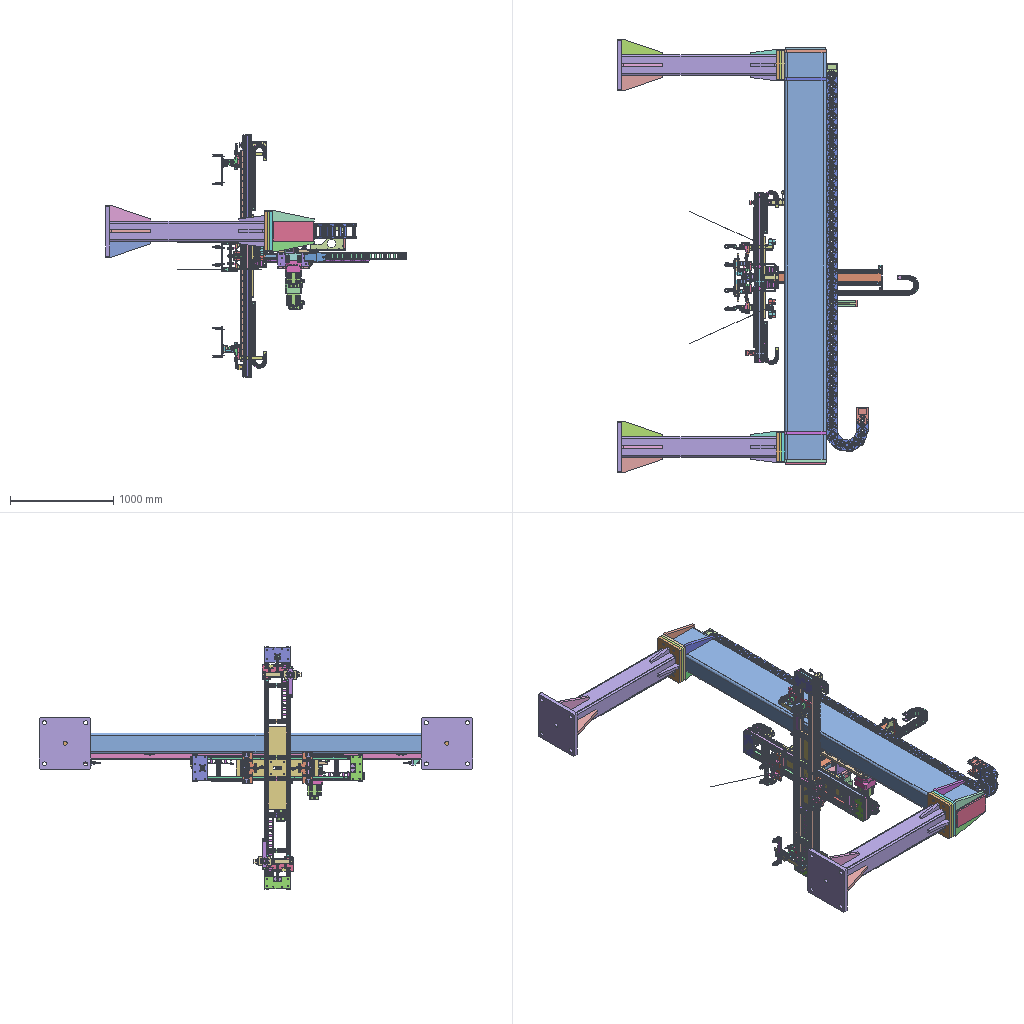Assembly | SolidWorks | 170 different items | 561 placed | box 2915 x 4200 x 2346 mm
Parts list (item | name | quantity | parent item | size | volume | features):
1 | (subassembly) | x2 | - | - | 1868083 mm3 | features InContextFeatHolder 12, ReferencePattern 4, CompositeCurve 2, MirrorCompFeat 1
2 | (subassembly) | x2 | - | - | 1438864 mm3 | features InContextFeatHolder 22, ReferencePattern 3, CompositeCurve 1, MirrorCompFeat 1
3 | (subassembly) | x1 | in 22 | 29 x 32 x 32 mm | 15807 mm3 | -
4 | (subassembly) | x1 | in 22 | 45 x 45 x 34 mm | 25485 mm3 | -
5 | (subassembly) | x1 | in 22 | 45 x 45 x 22 mm | 19865 mm3 | -
6 | (subassembly) | x4 | in 1 | 100.5 x 39 x 24.85 mm | 31183 mm3 | -
7 | (subassembly) | x2 | in 1 | 191 x 54 x 69 mm | 317476 mm3 | -
8 | (subassembly) | x2 | in 21 | 38.735 x 58.5 x 31.374 mm | 22045 mm3 | -
9 | (subassembly) | x2 | in 1 | 179.68 x 29.769 x 35.214 mm | 28072 mm3 | -
10 | (subassembly) | x1 | in 16 | 220 x 170 x 130 mm | 1941272 mm3 | -
11 | (subassembly) | x4 | in 2 | 17 x 70.5 x 19.048 mm | 7303 mm3 | -
12 | (subassembly) | x2 | in 22 | - | 654604 mm3 | -
13 | (subassembly) | x2 | in 22 | 72.4 x 145.352 x 414.628 mm | 469160 mm3 | -
14 | (subassembly) | x1 | in 21 | - | 1169113 mm3 | features ReferencePattern 9, LocalLPattern 1
15 | (subassembly) | x1 | in 20 | - | 15476828 mm3 | -
16 | (subassembly) | x1 | in 21 | 220 x 170 x 130 mm | 1941272 mm3 | -
17 | (subassembly) | x4 | in 2 | 100.5 x 39 x 24.85 mm | 31183 mm3 | -
18 | (subassembly) | x2 | in 2 | 179.229 x 29.769 x 35.214 mm | 28072 mm3 | -
19 | (subassembly) | x2 | in 20 | 26 x 157 x 29.132 mm | 41866 mm3 | -
20 | (subassembly) | x1 | - | - | 164128062 mm3 | features ReferencePattern 3, LocalLPattern 2
21 | (subassembly) | x1 | - | - | 39375353 mm3 | features InContextFeatHolder 40, ReferencePattern 26, LocalLPattern 4, LocalCirPattern 1, MirrorCompFeat 1
22 | (subassembly) | x1 | - | - | 17712446 mm3 | features ReferencePattern 14, InContextFeatHolder 8, Belt 2, LocalCirPattern 2, MirrorCompFeat 1, RefAxis 1
23 | (subassembly) | x4 | in 1 | 17 x 70.5 x 19.048 mm | 7303 mm3 | -
24 | - | x2 | in 18 | 116 x 21 x 21 mm | 16272 mm3 | features BaseBody 1, ICE 1, MoveCopyBody 1, Split 1
25 | - | x2 | in 21 | 23 x 18 x 900 mm | 312541 mm3 | features BaseBody 1, HoleWzd 1, ICE 1, MoveFace 1
26 | - | x4 | in 22 | 15 x 12.5 x 540 mm | 86755 mm3 | features BaseBody 1, HoleWzd 1, ICE 1, MoveFace 1
27 | - | x4 | in 20 | 23 x 18 x 1620 mm | 561456 mm3 | features MoveFace 3, BaseBody 1, HoleWzd 1
28 | - | x4 | in 22 | 15 x 12.5 x 1020 mm | 163723 mm3 | features BaseBody 1, HoleWzd 1, ICE 1, MoveFace 1
29 | - | x2 | in 1 | 34 x 19.5 x 56.8 mm | 30383 mm3 | features BaseBody 1
30 | - | x10 | in 21 | 48 x 26 x 82.6 mm | 80910 mm3 | features BaseBody 1
31 | - | x4 | in 1 | 12 x 42 x 42 mm | 9526 mm3 | features Revolution 5, CirPattern 2, RefAxis 1, RevCut 1
32 | - | x1 | in 21 | 160 x 160 x 283 mm | 4310215 mm3 | features ICE 18, CirPattern 4, Fillet 2, Revolution 2, Chamfer 1, RevCut 1
33 | - | x1 | in 21 | 160 x 160 x 330 mm | 5402193 mm3 | features ICE 18, CirPattern 4, Fillet 2, Revolution 2, Chamfer 1, RevCut 1
34 | - | x1 | in 22 | 54 x 54 x 34.8 mm | 31489 mm3 | features BaseBody 1
35 | - | x4 | in 11 | 12 x 70.5 x 12 mm | 6151 mm3 | features BaseBody 1
36 | - | x2 | in 22 | 60 x 60 x 115 mm | 222679 mm3 | features BaseBody 7
37 | - | x2 | in 8 | 31.47 x 20 x 31.374 mm | 10219 mm3 | features BaseBody 1
38 | - | x2 | in 8 | 33 x 58.5 x 20 mm | 11826 mm3 | features BaseBody 1
39 | - | x12 | in 6, 7 | 4 x 5.4 x 50 mm | 499.042 mm3 | features BaseBody 1
40 | - | x2 | in 9 | 6 x 25 x 22 mm | 1467 mm3 | features BaseBody 1
41 | - | x2 | in 9 | 5 x 11.547 x 10 mm | 331.011 mm3 | features BaseBody 1
42 | - | x2 | in 9 | 108 x 15.5 x 15.5 mm | 6247 mm3 | features BaseBody 1
43 | - | x2 | in 9 | 116 x 21 x 21 mm | 16272 mm3 | features BaseBody 1, ICE 1, MoveCopyBody 1, Split 1
44 | - | x2 | in 21 | 60 x 24 x 205 mm | 179716 mm3 | features BaseBody 1
45 | - | x4 | in 23 | 12 x 70.5 x 12 mm | 6151 mm3 | features BaseBody 1
46 | - | x8 | in 11 | 17 x 4 x 19.048 mm | 576.259 mm3 | features BaseBody 1
47 | - | x8 | in 23 | 17 x 4 x 19.048 mm | 576.259 mm3 | features BaseBody 1
48 | - | x2 | in 19 | 20 x 157 x 20 mm | 38514 mm3 | features BaseBody 1
49 | - | x4 | in 19 | 26 x 6 x 29.132 mm | 1676 mm3 | features BaseBody 1
50 | - | x4 | in 9 | 37.5 x 29.1 x 18.4 mm | 1877 mm3 | features BaseBody 1
51 | - | x1 | in 3 | 13.7 x 32 x 32 mm | 7455 mm3 | features BaseBody 1, ICE 1
52 | - | x1 | in 3 | 13.7 x 32 x 32 mm | 6989 mm3 | features BaseBody 1
53 | - | x1 | in 3 | 5.6 x 31 x 31 mm | 974.208 mm3 | features BaseBody 1
54 | - | x4 | in 3 | 9 x 5 x 5 mm | 97.086 mm3 | features BaseBody 1
55 | - | x1 | in 22 | 45 x 45 x 22 mm | 22602 mm3 | features ICE 4, BaseBody 1
56 | - | x1 | in 4 | 45 x 45 x 34 mm | 25485 mm3 | features BaseBody 1
57 | - | x4 | in 18 | 37.5 x 29.1 x 18.4 mm | 1877 mm3 | features BaseBody 1
58 | - | x4 | in 1, 2 | 33 x 6 x 36 mm | 5895 mm3 | features ICE 2, MoveFace 2, BaseBody 1, HoleWzd 1
59 | - | x2 | in 5, 22 | 45 x 45 x 22 mm | 19865 mm3 | features BaseBody 1, RefAxis 1
60 | - | x4 | in 6 | 50 x 39 x 23.5 mm | 27612 mm3 | features BaseBody 1
61 | - | x4 | in 6 | 21 x 15.4 x 10.1 mm | 1286 mm3 | features BaseBody 1
62 | - | x4 | in 6 | 21 x 15.4 x 10.1 mm | 1286 mm3 | features BaseBody 1
63 | - | x2 | in 7 | 169 x 54 x 69 mm | 316478 mm3 | features BaseBody 1
64 | - | x2 | in 10, 21 | 220 x 170 x 130 mm | 1941272 mm3 | features BaseBody 1
65 | - | x54 | in 12, 13 | 68 x 35.356 x 81.35 mm | 37089 mm3 | features BaseBody 1
66 | - | x23 | in 14 | 72.6 x 45.28 x 91.28 mm | 47406 mm3 | features BaseBody 1
67 | - | x40 | in 15 | 145 x 107 x 206.999 mm | 368273 mm3 | features BaseBody 1
68 | - | x4 | in 17 | 50 x 39 x 23.5 mm | 27612 mm3 | features BaseBody 1
69 | - | x4 | in 12, 13 | 72.4 x 35.35 x 67.662 mm | 29898 mm3 | features BaseBody 1
70 | - | x4 | in 12, 13 | 72.4 x 35.35 x 67.664 mm | 31284 mm3 | features BaseBody 1
71 | - | x1 | in 14 | 73.47 x 44.999 x 83.497 mm | 38091 mm3 | features BaseBody 1
72 | - | x1 | in 14 | 73.47 x 44.999 x 83.497 mm | 40679 mm3 | features BaseBody 1
73 | - | x1 | in 15 | 144 x 107 x 180 mm | 372084 mm3 | features BaseBody 1
74 | - | x1 | in 15 | 144 x 107 x 180 mm | 373805 mm3 | features BaseBody 1
75 | - | x2 | in 1 | 50 x 50 x 10 mm | 14543 mm3 | features BaseBody 1, RefAxis 1
76 | - | x2 | in 1 | 50 x 12 x 10 mm | 5397 mm3 | features BaseBody 1, HoleWzd 1, ICE 1
77 | - | x4 | in 17 | 21 x 15.4 x 10.1 mm | 1286 mm3 | features BaseBody 1
78 | - | x4 | in 17 | 21 x 15.4 x 10.1 mm | 1286 mm3 | features BaseBody 1
79 | - | x2 | in 2 | 50 x 50 x 10 mm | 14543 mm3 | features BaseBody 1, RefAxis 1
80 | - | x2 | in 2 | 50 x 12 x 10 mm | 5397 mm3 | features BaseBody 1, HoleWzd 1, ICE 1
81 | - | x1 | in 21 | 142 x 202 x 99 mm | 619754 mm3 | features BaseBody 1
82 | - | x1 | in 20 | 2009 x 24 x 24 mm | 1024177 mm3 | features ICE 10, BaseBody 1, LPattern 1, MoveFace 1
83 | - | x8 | in 21 | - | - | features RefSurface 9
84 | - | x4 | in 21 | - | - | features RefSurface 9
85 | - | x2 | in 21 | 13.344 x 9 x 13.344 mm | 1017 mm3 | features BaseBody 1
86 | - | x2 | in 21 | - | - | features RefSurface 1
87 | - | x2 | in 20 | 1570 x 500 x 500 mm | 29641235 mm3 | features ICE 3, Chamfer 2, CirPattern 2, HoleWzd 2, Split 2, CombineBodies 1, Rib 1, WeldMemberFeat 1, WeldmentFeature 1
88 | - | x1 | in 20 | 4040 x 400 x 430 mm | 79794691 mm3 | features HoleWzd 6, ICE 4, MirrorSolid 3, Chamfer 2, EndCap 2, Cut 1, MirrorPattern 1, WeldMemberFeat 1, WeldmentFeature 1
89 | - | x2 | in 20 | 300 x 20 x 400 mm | 2385381 mm3 | features Chamfer 1, Extrusion 1, HoleWzd 1
90 | - | x2 | in 20 | 90 x 100 x 110 mm | 460863 mm3 | features HoleWzd 3, ICE 2, Extrusion 1, MirrorSolid 1
91 | - | x2 | in 20 | 28 x 5 x 100 mm | 4922 mm3 | features BossThin 1, ExtruThin 1, HoleWzd 1, MirrorSolid 1
92 | - | x1 | in 21 | 600 x 25 x 300 mm | 3745145 mm3 | features HoleWzd 11, Cut 2, Chamfer 1, Extrusion 1
93 | - | x2 | in 20, 21 | 1008 x 24 x 24 mm | 511477 mm3 | features BaseBody 1
94 | - | x1 | in 21 | 248 x 60 x 12 mm | 176365 mm3 | features HoleWzd 2, Chamfer 1, Extrusion 1
95 | - | x1 | in 21 | 25 x 60 x 12 mm | 15515 mm3 | features HoleWzd 2, Chamfer 1, Extrusion 1
96 | - | x1 | in 21 | 25 x 98 x 142 mm | 49886 mm3 | features HoleWzd 2, BreakCorner 1, FlatPattern 1, SMBaseFlange 1, SheetMetal 1
97 | - | x1 | in 21 | 300 x 25 x 300 mm | 1546097 mm3 | features HoleWzd 9, Cut 2, Chamfer 1, Extrusion 1
98 | - | x2 | in 21 | 200 x 180 x 12 mm | 261071 mm3 | features HoleWzd 4, MirrorPattern 2, Chamfer 1, Cut 1, Extrusion 1
99 | - | x2 | in 21 | 50 x 25 x 15 mm | 15237 mm3 | features HoleWzd 2, Chamfer 1, Extrusion 1
100 | - | x1 | in 21 | 1125 x 200 x 236 mm | 3630332 mm3 | features ICE 7, HoleWzd 5, Chamfer 2, Fillet 2, Cut 1, EndCap 1, MirrorPattern 1, MoveFace 1, WeldMemberFeat 1, WeldmentFeature 1
101 | - | x2 | in 21 | 50 x 25 x 15 mm | 15782 mm3 | features Chamfer 1, Extrusion 1, HoleWzd 1
102 | - | x1 | in 21 | 800 x 20 x 800 mm | 6619888 mm3 | features HoleWzd 3, Chamfer 1, Cut 1, Extrusion 1, Fillet 1
103 | - | x1 | in 21 | 135 x 25 x 300 mm | 964423 mm3 | features HoleWzd 3, Cut 1, Extrusion 1, MirrorPattern 1
104 | - | x4 | in 2 | 34 x 19.5 x 56.8 mm | 30383 mm3 | features BaseBody 1
105 | - | x1 | in 21 | 135 x 25 x 300 mm | 964423 mm3 | features MirrorStock 1
106 | - | x1 | in 21 | 340 x 60 x 12 mm | 241410 mm3 | features HoleWzd 3, Chamfer 1, Extrusion 1
107 | - | x1 | in 21 | 80 x 75 x 10 mm | 45981 mm3 | features HoleWzd 2, Chamfer 1, Cut 1, Extrusion 1
108 | - | x1 | in 21 | 248 x 323 x 12 mm | 393029 mm3 | features HoleWzd 2, ICE 2, Extrusion 1, Fillet 1
109 | - | x2 | in 21 | 25 x 34.5 x 20 mm | 1892 mm3 | features BreakCorner 1, FlatPattern 1, HoleWzd 1, ICE 1, SMBaseFlange 1, SheetMetal 1
110 | - | x1 | in 21 | 15 x 62.5 x 20 mm | 2923 mm3 | features BreakCorner 1, FlatPattern 1, HoleWzd 1, SMBaseFlange 1, SheetMetal 1
111 | - | x1 | in 21 | 28 x 5 x 800 mm | 39502 mm3 | features BossThin 1, ExtruThin 1, HoleWzd 1, MirrorSolid 1
112 | - | x1 | in 21 | 12 x 37 x 20 mm | 1356 mm3 | features BreakCorner 1, FlatPattern 1, HoleWzd 1, SMBaseFlange 1, SheetMetal 1
113 | - | x1 | in 21 | 25 x 25 x 13 mm | 5523 mm3 | features Extrusion 1, HoleWzd 1
114 | - | x4 | in 22 | 540 x 12 x 40 mm | 251867 mm3 | features HoleWzd 3, LPattern 2, Chamfer 1, Extrusion 1
115 | - | x4 | in 2 | 12 x 42 x 42 mm | 9526 mm3 | features Revolution 5, CirPattern 2, RefAxis 1, RevCut 1
116 | - | x4 | in 22 | 1020 x 20 x 40 mm | 797316 mm3 | features HoleWzd 3, LPattern 2, Chamfer 1, Extrusion 1
117 | - | x1 | in 22 | - | 6888889 mm3 | features WeldMemberFeat 1, WeldmentFeature 1
118 | - | x2 | in 22 | 250 x 12 x 117.5 mm | 341494 mm3 | features HoleWzd 4, Chamfer 1, Extrusion 1
119 | - | x1 | in 22 | 50 x 34 x 12 mm | 19690 mm3 | features Extrusion 1, HoleWzd 1, MirrorPattern 1
120 | - | x2 | in 22 | 50 x 79 x 12 mm | 40495 mm3 | features HoleWzd 3, Chamfer 1, Extrusion 1
121 | - | x4 | in 22 | 10 x 10 x 70 mm | 5498 mm3 | features Extrusion 1
122 | - | x2 | in 22 | 50 x 74 x 12 mm | 31467 mm3 | features Extrusion 1, HoleWzd 1, ICE 1, MirrorPattern 1
123 | - | x2 | in 22 | 250 x 12 x 145 mm | 416706 mm3 | features Cut 2, HoleWzd 2, Chamfer 1, Extrusion 1
124 | - | x1 | in 22 | 10 x 10 x 58 mm | 4483 mm3 | features ICE 2, MirrorPattern 2, Extrusion 1, RefAxis 1
125 | - | x1 | in 22 | 50 x 34 x 12 mm | 19690 mm3 | features Extrusion 1, HoleWzd 1, MirrorPattern 1
126 | - | x8 | in 17 | 4 x 5.4 x 50 mm | 499.042 mm3 | features BaseBody 1
127 | - | x1 | in 22 | 10 x 10 x 98 mm | 7613 mm3 | features ICE 2, MirrorPattern 2, Extrusion 1, RefAxis 1
128 | - | x8 | in 22 | 40 x 3 x 80 mm | 9527 mm3 | features Fillet 2, Extrusion 1
129 | - | x1 | in 22 | 16 x 16 x 87 mm | 9059 mm3 | features ICE 2, Extrusion 1, HoleWzd 1, Revolution 1
130 | - | x4 | in 1 | 25 x 10 x 25 mm | 3874 mm3 | features HoleWzd 2, Chamfer 1, Extrusion 1
131 | - | x2 | in 1 | 26 x 80 x 22 mm | 22644 mm3 | features Chamfer 2, Cut 2, Extrusion 1, HoleWzd 1, ICE 1, MirrorPattern 1
132 | - | x4 | in 1 | 35 x 60 x 40 mm | 35844 mm3 | features Chamfer 2, HoleWzd 2, Extrusion 1, ICE 1
133 | - | x2 | in 1 | 80 x 300 x 12 mm | 155894 mm3 | features Cut 3, HoleWzd 3, Chamfer 2, CirPattern 1, Extrusion 1, Fillet 1
134 | - | x2 | in 1 | 80 x 333.5 x 12 mm | 174640 mm3 | features Chamfer 2, Cut 2, HoleWzd 2, Extrusion 1, Fillet 1
135 | - | x2 | in 1 | 46 x 15 x 50 mm | 17863 mm3 | features Chamfer 4, Extrusion 1, HoleWzd 1, ICE 1
136 | - | x2 | in 1 | 20 x 50 x 10 mm | 7631 mm3 | features Chamfer 1, Extrusion 1, HoleWzd 1
137 | - | x2 | in 18 | 6 x 25 x 22 mm | 1467 mm3 | features BaseBody 1
138 | - | x2 | in 1 | 20 x 235 x 20 mm | 73572 mm3 | features ICE 3, Chamfer 1, Extrusion 1
139 | - | x4 | in 1 | 95 x 20 x 80 mm | 71658 mm3 | features ICE 2, Chamfer 1, Extrusion 1, Fillet 1, HoleWzd 1
140 | - | x4 | in 1 | 15 x 35 x 40 mm | 15250 mm3 | features Chamfer 1, Extrusion 1, HoleWzd 1
141 | - | x4 | in 1 | 27 x 35 x 80 mm | 44069 mm3 | features Chamfer 2, HoleWzd 2, Extrusion 1, ICE 1
142 | - | x4 | in 1 | 35 x 12 x 34.943 mm | 6766 mm3 | features HoleWzd 2, Chamfer 1, Extrusion 1, ICE 1, MirrorPattern 1
143 | - | x2 | in 1 | 30 x 37.5 x 36 mm | 19999 mm3 | features HoleWzd 2, Chamfer 1, ExtruThin 1
144 | - | x8 | in 1 | 17.5 x 30 x 12 mm | 2171 mm3 | features Extrusion 1, Fillet 1, HoleWzd 1, ICE 1
145 | - | x4 | in 1, 2 | 113 x 30 x 232 mm | 30522 mm3 | features BreakCorner 1, FlatPattern 1, SMBaseFlange 1, SheetMetal 1
146 | - | x4 | in 1 | 35 x 35 x 20 mm | 13186 mm3 | features HoleWzd 3, Chamfer 1, Extrusion 1, ICE 1
147 | - | x2 | in 1 | 300 x 140 x 20 mm | 458590 mm3 | features HoleWzd 8, Chamfer 5, Cut 4, Fillet 4, ICE 3, Extrusion 1
148 | - | x2 | in 18 | 5 x 11.547 x 10 mm | 331.011 mm3 | features BaseBody 1
149 | - | x5 | in 1, 21 | 25 x 25 x 23 mm | 9481 mm3 | features Extrusion 1, HoleWzd 1
150 | - | x4 | in 2 | 35 x 35 x 20 mm | 13186 mm3 | features HoleWzd 3, Chamfer 1, Extrusion 1, ICE 1
151 | - | x2 | in 2 | 20 x 50 x 10 mm | 7631 mm3 | features Chamfer 1, Extrusion 1, HoleWzd 1
152 | - | x2 | in 2 | 46 x 15 x 50 mm | 17863 mm3 | features Chamfer 4, Extrusion 1, HoleWzd 1, ICE 1
153 | - | x2 | in 2 | 26 x 80 x 22 mm | 22644 mm3 | features Chamfer 2, Cut 2, Extrusion 1, HoleWzd 1, ICE 1, MirrorPattern 1
154 | - | x2 | in 2 | 20 x 300 x 20 mm | 93992 mm3 | features ICE 3, Chamfer 1, Extrusion 1
155 | - | x2 | in 2 | 300 x 140 x 20 mm | 435356 mm3 | features HoleWzd 7, Chamfer 4, Cut 4, Fillet 3, ICE 2, Extrusion 1
156 | - | x2 | in 2 | 40 x 300 x 12 mm | 108008 mm3 | features Cut 3, Chamfer 2, HoleWzd 2, ICE 2, Extrusion 1, Fillet 1
157 | - | x4 | in 2 | 35 x 56.7 x 40 mm | 34458 mm3 | features Chamfer 2, HoleWzd 2, Extrusion 1, ICE 1
158 | - | x2 | in 2 | 30 x 37.5 x 36 mm | 19999 mm3 | features HoleWzd 2, Chamfer 1, ExtruThin 1
159 | - | x2 | in 18 | 108 x 15.5 x 15.5 mm | 6247 mm3 | features BaseBody 1
160 | - | x4 | in 2 | 35 x 12 x 34.943 mm | 6766 mm3 | features HoleWzd 2, Chamfer 1, Extrusion 1, ICE 1, MirrorPattern 1
161 | - | x4 | in 2 | 15 x 35 x 40 mm | 15250 mm3 | features Chamfer 1, Extrusion 1, HoleWzd 1
162 | - | x4 | in 2 | 95 x 20 x 80 mm | 71658 mm3 | features ICE 2, Chamfer 1, Extrusion 1, Fillet 1, HoleWzd 1
163 | - | x4 | in 2 | 56.8 x 38 x 28 mm | 56349 mm3 | features Chamfer 1, Cut 1, Extrusion 1
164 | - | x4 | in 2 | 27 x 35 x 80 mm | 44069 mm3 | features Chamfer 2, HoleWzd 2, Extrusion 1, ICE 1
165 | - | x8 | in 2 | 17.5 x 30 x 12 mm | 2171 mm3 | features Extrusion 1, Fillet 1, HoleWzd 1, ICE 1
166 | - | x8 | in 21 | - | - | features RefSurface 2
167 | - | x2 | in 22 | 63.089 x 175.904 x 146.235 mm | 489456 mm3 | features BaseBody 2
168 | - | x3 | in 20 | 26.2 x 15.5 x 20.7 mm | 2180 mm3 | features BaseBody 1
169 | - | x1 | in 21 | 26.2 x 15.5 x 20.7 mm | 2180 mm3 | features BaseBody 1
170 | - | x2 | in 21 | 100 x 100 x 76 mm | 350240 mm3 | features ICE 3, Chamfer 2, CirPattern 2, HoleWzd 1, RefAxis 1, Revolution 1
Mates (type | each side: item.copy, entity, surface, feature), first 385 of 538 lines:
In the top assembly
Width | 155.1 face plane Boss-Extrude 1 | 155.1 face plane Boss-Extrude 1 | 117.1 face plane Aluminium Profile 40 X 80L X R0.3(1) | 117.1 face plane Aluminium Profile 40 X 80L X R0.3(1)
Coincident | 26.1 face plane 输入1 | 104.1 face plane 输入1
DistanceDim | assembly plane | 87.1 face plane Boss-Extrude 1
DistanceDim | assembly plane | 87.1 face plane Gb/6728-1986方形空心型钢 200 X 200 X 10(1)
Parallel | 88.1 face plane Gb/6728-1986矩形空心型钢 400 X 200 X 12(1) | assembly plane
Width | 30.1 face plane 输入1 | 30.1 face plane 输入1 | 27.1 face plane 输入1 | 27.1 face plane 输入1
Width | 30.2 face plane 输入1 | 30.2 face plane 输入1 | 27.2 face plane 输入1 | 27.2 face plane 输入1
Coincident | 102.1 face plane Boss-Extrude 1 | 117.1 face plane Aluminium Profile 40 X 80L X R0.3(1)
Width | 117.1 face plane Aluminium Profile 40 X 80L X R0.3(1) | 117.1 face plane Aluminium Profile 40 X 80L X R0.3(1) | 102.1 face plane Boss-Extrude 1 | 102.1 face plane Boss-Extrude 1 | 2 times
Parallel | 82.1 face plane 输入1 | 8.1 plane
LimitDistanceDim | 92.1 face plane Boss-Extrude 1 | 88.1 face plane Boss-Extrude 3
LimitDistanceDim | 155.2 face plane Boss-Extrude 1 | 123.1 face plane Boss-Extrude 1
Parallel | assembly face | 87.1 face plane Boss-Extrude 1
Width | assembly face | assembly face | 117.1 face plane Aluminium Profile 40 X 80L X R0.3(1) | 117.1 face plane Aluminium Profile 40 X 80L X R0.3(1) | 2 times
Coincident | 28.1 face plane 输入1 | 29.1 face plane 输入1
Width | 147.1 face plane Boss-Extrude 1 | 147.1 face plane Boss-Extrude 1 | 116.1 face plane Boss-Extrude 1 | 116.2 face plane Boss-Extrude 1
LimitDistanceDim | 147.1 face plane Boss-Extrude 1 | 116.1 face plane Boss-Extrude 1
Coincident | 87.1 face plane Gb/6728-1986方形空心型钢 200 X 200 X 10(1) | assembly plane
Coincident | 27.1 face plane 输入1 | 30.1 face plane 输入1
In subassembly 1
Coincident | 147.2 face plane Cut-Extrude 2 | 143.1 face plane Extrude-薄壁1
Width | 147.2 face plane Boss-Extrude 1 | 147.2 face plane Boss-Extrude 1 | 143.1 face plane Extrude-薄壁1 | 143.1 face plane Extrude-薄壁1
DistanceDim | 143.1 face plane Extrude-薄壁1 | 147.2 face plane Boss-Extrude 1
Coincident | 29.2 face plane 输入1 | 147.2 face plane Cut-Extrude 1
Width | 143.1 face plane Extrude-薄壁1 | 143.1 face plane Extrude-薄壁1 | 58.1 face plane 输入1 | 58.1 face plane 输入1
Width | 29.2 face plane 输入1 | 29.2 face plane 输入1 | 147.2 face plane Cut-Extrude 1 | 147.2 face plane Cut-Extrude 1
Width | 147.2 face plane Boss-Extrude 1 | 147.2 face plane Boss-Extrude 1 | 29.2 face plane 输入1 | 29.2 face plane 输入1
DistanceDim | 58.1 face plane 输入1 | 143.1 face plane Extrude-薄壁1
DistanceDim | 58.1 face plane 输入1 | 147.2 face plane Cut-Extrude 2
Coincident | 147.2 face plane Boss-Extrude 1 | 145.1 face plane Base-Flange 1 | 2 times
Parallel | 147.2 face plane Boss-Extrude 1 | 145.1 face plane Base-Flange 1
Coincident | 135.1 face plane Boss-Extrude 1 | 136.1 face plane Boss-Extrude 1
Width | 135.1 face plane Boss-Extrude 2 | 135.1 face plane Boss-Extrude 2 | 136.1 face plane Boss-Extrude 1 | 136.1 face plane Boss-Extrude 1
Coincident | 131.1 face plane Cut-Extrude 2 | 43.1 face plane 输入1
Concentric | 131.1 face cylinder Cut-Extrude 1 | 43.1 face cylinder 输入1
Coincident | 41.1 face plane 输入1 | 136.1 face plane Boss-Extrude 1
Width | 136.1 face plane Boss-Extrude 1 | 136.1 face plane Boss-Extrude 1 | 42.1 face cylinder 输入1
Coincident | 136.1 face plane Boss-Extrude 1 | 76.1 face plane 输入1 | 2 times
Width | 136.1 face plane Boss-Extrude 1 | 136.1 face plane Boss-Extrude 1 | 76.1 face plane 输入1 | 76.1 face plane 输入1
DistanceDim | 75.1 axis | 136.1 face plane Boss-Extrude 1
RackPinionDim | 76.1 select_type:24 | 75.1 select_type:24
Concentric | 138.1 face cylinder Boss-Extrude 1 | 75.1 face cylinder 输入1
Concentric | 138.1 face cylinder Boss-Extrude 1 | 31.1 face cylinder Revolve 1
Concentric | 138.1 face cylinder Boss-Extrude 1 | 139.1 face cylinder Boss-Extrude 1
Concentric | 138.1 face cylinder Boss-Extrude 1 | 140.1 face cylinder Boss-Extrude 1
Concentric | 138.1 face cylinder Boss-Extrude 1 | 141.1 face cylinder Boss-Extrude 1
Concentric | 138.1 face cylinder Boss-Extrude 1 | 140.2 face cylinder Boss-Extrude 1
Concentric | 138.1 face cylinder Boss-Extrude 1 | 141.2 face cylinder Boss-Extrude 1
Coincident | 138.1 face plane ZJCQC | 75.1 face plane 输入1
Concentric | 138.1 face cylinder Boss-Extrude 1 | 142.1 face cylinder Boss-Extrude 1
Concentric | 138.1 face cylinder Boss-Extrude 1 | 142.2 face cylinder Boss-Extrude 1
PlanarAngleDim | 138.1 plane | 141.2 face plane Boss-Extrude 1
Coincident | 138.1 face plane Boss-Extrude 1 | 141.2 face plane Boss-Extrude 1
Coincident | 132.1 face plane Boss-Extrude 1 | 134.1 face plane Boss-Extrude 1 | 2 times
Coincident | 132.1 face plane Boss-Extrude 1 | 141.2 face plane Cut-Extrude 1 | 2 times
Coincident | 134.1 face plane Boss-Extrude 1 | 63.1 face plane 输入1
Width | 134.1 face plane Boss-Extrude 1 | 134.1 face plane Boss-Extrude 1 | 63.1 face plane 输入1 | 63.1 face plane 输入1
DistanceDim | 63.1 face plane 输入1 | 133.1 face plane Boss-Extrude 1
Coincident | 133.1 face plane Boss-Extrude 1 | 60.1 face plane 输入1
Width | 133.1 face plane Cut-Extrude 2 | 133.1 face plane Cut-Extrude 2 | 60.2 face plane 输入1 | 60.2 face plane 输入1
DistanceDim | 60.2 face plane 输入1 | 133.1 face plane Boss-Extrude 1
Width | 133.1 face plane Cut-Extrude 2 | 133.1 face plane Cut-Extrude 2 | 60.1 face plane 输入1 | 60.1 face plane 输入1
DistanceDim | 133.1 face plane Boss-Extrude 1 | 60.1 face plane 输入1
Coincident | 60.1 face plane 输入1 | 60.2 face plane 输入1
Coincident | 61.1 face plane 输入1 | 144.1 face plane Boss-Extrude 1
Width | 61.1 face plane 输入1 | 61.1 face plane 输入1 | 144.1 face plane Boss-Extrude 1 | 144.1 face plane Boss-Extrude 1
Coincident | 61.1 face plane 输入1 | 144.1 face plane Cut-Extrude 1
Coincident | 62.1 face plane 输入1 | 144.2 face plane Cut-Extrude 1
Width | 144.2 face plane Boss-Extrude 1 | 144.2 face plane Boss-Extrude 1 | 62.1 face plane 输入1 | 62.1 face plane 输入1
Coincident | 62.2 face plane 输入1 | 144.3 face plane Cut-Extrude 1
Width | 144.3 face plane Boss-Extrude 1 | 144.3 face plane Boss-Extrude 1 | 62.2 face plane 输入1 | 62.2 face plane 输入1
Coincident | 61.2 face plane 输入1 | 144.4 face plane Cut-Extrude 1
Coincident | 62.2 face plane 输入1 | 144.3 face plane Boss-Extrude 1
Width | 144.4 face plane Boss-Extrude 1 | 144.4 face plane Boss-Extrude 1 | 61.2 face plane 输入1 | 61.2 face plane 输入1
Coincident | 132.2 face plane Boss-Extrude 1 | 141.1 face plane Cut-Extrude 1 | 2 times
Coincident | 132.2 face plane Boss-Extrude 1 | 141.1 face plane Boss-Extrude 1
Coincident | 75.1 face plane 输入1 | 142.1 face plane Boss-Extrude 1
Coincident | 75.1 face plane 输入1 | 142.2 face plane Boss-Extrude 1
Parallel | 75.1 plane | 142.1 face plane Cut-Extrude 1
Concentric | 31.1 face cylinder Revolve 1 | 139.2 face cylinder Boss-Extrude 1
Coincident | 31.1 face plane Revolve 1 | 139.2 face plane Boss-Extrude 2
Concentric | 139.1 face cylinder Boss-Extrude 1 | 31.2 face cylinder Revolve 1
Coincident | 139.1 face plane Boss-Extrude 2 | 31.2 face plane Revolve 1
Parallel | 140.1 face plane Boss-Extrude 1 | 141.1 face plane Boss-Extrude 1
Coincident | 140.2 face plane Boss-Extrude 1 | 141.2 face plane Boss-Extrude 1 | 2 times
Coincident | 142.1 face plane Mirror 1 | 142.2 face plane Mirror 1
Coincident | 47.1 face plane 输入1 | 146.1 face plane Boss-Extrude 1
Coincident | 144.1 face plane Boss-Extrude 1 | 144.2 face plane Boss-Extrude 1
Coincident | 144.3 face plane Boss-Extrude 1 | 144.4 face plane Boss-Extrude 1
Coincident | 147.2 face plane Boss-Extrude 1 | 135.1 face plane Boss-Extrude 1
Coincident | 135.1 face plane Boss-Extrude 1 | 147.2 face plane Cut-Extrude 4
Coincident | 131.1 face plane Mirror 1 | 147.2 face plane Boss-Extrude 2
Parallel | 147.2 face plane Boss-Extrude 1 | 139.2 face plane Boss-Extrude 1
Parallel | 147.2 face plane Boss-Extrude 1 | 139.1 face plane Boss-Extrude 1
Coincident | 147.2 face plane Boss-Extrude 1 | 146.1 face plane Boss-Extrude 1
Coincident | 146.1 face plane Boss-Extrude 1 | 147.2 face plane Boss-Extrude 1
Coincident | 139.1 face plane Boss-Extrude 1 | 147.2 face plane Boss-Extrude 1
Coincident | 139.1 face plane Boss-Extrude 1 | 147.2 face plane Cut-Extrude 4
Coincident | 139.2 face plane Boss-Extrude 1 | 147.2 face plane Cut-Extrude 4
Coincident | 139.2 face plane Boss-Extrude 1 | 147.2 face plane Boss-Extrude 1
Coincident | 131.1 face plane Boss-Extrude 1 | 147.2 face plane Cut-Extrude 3
DistanceDim | 131.1 face plane Boss-Extrude 1 | 139.1 face plane Boss-Extrude 1
Coincident | 139.1 face plane Boss-Extrude 1 | 146.1 face plane Boss-Extrude 1
DistanceDim | 63.1 face plane 输入1 | 132.1 face plane Boss-Extrude 1
Coincident | 140.1 face plane Boss-Extrude 1 | 141.1 face plane Boss-Extrude 1
Coincident | 132.1 face plane Boss-Extrude 1 | 141.2 face plane Boss-Extrude 1
DistanceDim | 140.1 face plane Boss-Extrude 1 | 139.2 face plane Boss-Extrude 1
DistanceDim | 147.2 face plane Boss-Extrude 1 | 138.1 face plane Boss-Extrude 1
Width | 134.1 face plane Boss-Extrude 1 | 134.1 face plane Boss-Extrude 1 | 132.1 face plane Boss-Extrude 2 | 132.1 face plane Boss-Extrude 1
Coincident | 132.1 face plane Boss-Extrude 1 | 132.2 face plane Boss-Extrude 1
Width | 139.2 face plane Boss-Extrude 1 | 139.1 face plane Boss-Extrude 1 | 75.1 face plane 输入1 | 75.1 face plane 输入1
Parallel | 132.2 face plane Boss-Extrude 1 | 147.2 face plane Boss-Extrude 1
Concentric | 63.1 face cylinder 输入1 | 133.1 edge
Parallel | 134.1 face plane Boss-Extrude 1 | 133.1 face plane Cut-Extrude 2
Coincident | 147.2 face plane Boss-Extrude 3 | 145.1 face plane Base-Flange 1
Coincident | 147.2 face plane Boss-Extrude 1 | 130.1 face plane Boss-Extrude 1 | 2 times
Width | 139.2 face plane Boss-Extrude 1 | 146.2 face plane Boss-Extrude 1 | 130.1 face plane Boss-Extrude 1 | 130.1 face plane Boss-Extrude 1
Concentric | 130.1 face cylinder M6 Tapped Hole 1 | 149.1 face cylinder M6 六角圆柱头Screw的柱形沉头Hole 1
Coincident | 130.1 face plane Boss-Extrude 1 | 149.1 face plane Boss-Extrude 1
In subassembly 23
Concentric | 45.1 face cylinder 输入1 | 47.2 face cylinder 输入1
Concentric | 45.1 face cylinder 输入1 | 47.3 face cylinder 输入1
In subassembly 9
LimitDistanceDim | 42.2 face plane 输入1 | 43.2 face plane 输入1
Concentric | 43.2 face cylinder 输入1 | 42.2 face cylinder 输入1
Concentric | 42.2 face cylinder 输入1 | 41.2 face cylinder 输入1
DistanceDim | 41.2 face plane 输入1 | 42.2 face plane 输入1
Concentric | 43.2 face cylinder 输入1 | 40.1 face cylinder 输入1
DistanceDim | 40.1 face plane 输入1 | 43.2 face plane 输入1
Parallel | 40.1 face plane 输入1 | 50.1 face plane 输入1
Parallel | 42.2 face plane 输入1 | 50.1 face plane 输入1
Parallel | 41.2 face plane 输入1 | 50.1 face plane 输入1
In subassembly 21
Coincident | 30.3 face plane 输入1 | 30.4 face plane 输入1
Coincident | 30.3 face plane 输入1 | 92.2 face plane Boss-Extrude 1
Parallel | 92.2 face plane Boss-Extrude 1 | 32.1 face plane Boss-Extrude 1
Width | 92.2 face plane Boss-Extrude 1 | 92.2 face plane Boss-Extrude 1 | 32.1 face plane Boss-Extrude 1 | 32.1 face plane Boss-Extrude 1
Coincident | 92.2 face plane Boss-Extrude 1 | 103.1 face plane Boss-Extrude 1
Parallel | 92.2 face plane Boss-Extrude 1 | 103.1 face plane Boss-Extrude 1
Width | 103.1 face plane Boss-Extrude 1 | 103.1 face plane Boss-Extrude 1 | 92.2 face plane Boss-Extrude 1 | 92.2 face plane Boss-Extrude 1
Coincident | 92.2 face plane Boss-Extrude 1 | 105.1 face plane | 3 times
DistanceDim | 32.1 face plane Boss-Extrude 1 | 92.2 face plane Boss-Extrude 1
Coincident | 92.2 face plane Boss-Extrude 1 | 98.1 face plane Boss-Extrude 1
Width | 92.2 face plane Cut-Extrude 1 | 92.2 face plane Cut-Extrude 1 | 101.1 face plane Boss-Extrude 1 | 101.1 face plane Boss-Extrude 1
Coincident | 92.2 face plane Boss-Extrude 1 | 99.1 face plane Boss-Extrude 1
DistanceDim | 92.2 face plane Boss-Extrude 1 | 99.1 face plane Boss-Extrude 1
Coincident | 92.2 face plane Boss-Extrude 1 | 95.1 face plane Boss-Extrude 1 | 2 times
DistanceDim | 92.2 face plane Boss-Extrude 1 | 95.1 face plane Boss-Extrude 1
Concentric | 64.1 face cylinder 输入1 | 32.1 face cylinder Cut-Revolve 1
Coincident | 64.1 face plane 输入1 | 32.1 face plane Boss-Extrude 3
Parallel | 64.1 face plane 输入1 | 32.1 face plane Boss-Extrude 3
Concentric | 32.1 face cylinder Revolve 1 | 170.1 face cylinder Revolve 1
Coincident | 32.1 face plane Boss-Extrude 1 | 98.1 face plane Boss-Extrude 1
Width | 98.1 face plane Boss-Extrude 1 | 98.1 face plane Boss-Extrude 1 | 32.1 face plane Boss-Extrude 1 | 32.1 face plane Boss-Extrude 1
Width | 32.1 face plane Boss-Extrude 1 | 32.1 face plane Boss-Extrude 1 | 98.1 face plane Boss-Extrude 1 | 98.1 face plane Boss-Extrude 1
Coincident | 103.1 face plane Boss-Extrude 1 | 97.1 face plane Boss-Extrude 1
Width | 103.1 face plane Boss-Extrude 1 | 103.1 face plane Boss-Extrude 1 | 97.1 face plane Boss-Extrude 1 | 97.1 face plane Boss-Extrude 1
DistanceDim | 30.5 face plane 输入1 | 103.1 face plane Boss-Extrude 1 | 2 times
DistanceDim | 30.6 face plane 输入1 | 103.1 face plane Boss-Extrude 1
DistanceDim | 72.1 face plane 输入1 | 103.1 face plane Boss-Extrude 1
Coincident | 103.1 face plane Boss-Extrude 1 | 107.1 face plane Boss-Extrude 1 | 2 times
Parallel | 97.1 face plane Boss-Extrude 1 | 100.1 face plane Boss-Extrude 3
Parallel | 97.1 face plane Boss-Extrude 1 | 33.1 face plane Boss-Extrude 1
Width | 97.1 face plane Boss-Extrude 1 | 97.1 face plane Boss-Extrude 1 | 33.1 face plane Boss-Extrude 1 | 33.1 face plane Boss-Extrude 1
Coincident | 97.1 face plane Boss-Extrude 1 | 98.2 face plane Boss-Extrude 1
Width | 97.1 face plane Cut-Extrude 1 | 97.1 face plane Cut-Extrude 1 | 101.2 face plane Boss-Extrude 1 | 101.2 face plane Boss-Extrude 1
Coincident | 97.1 face plane Boss-Extrude 1 | 99.2 face plane Boss-Extrude 1
Coincident | 97.1 face plane Cut-Extrude 1 | 99.2 face plane Boss-Extrude 1
Coincident | 100.1 face plane Boss-Extrude 1 | 25.1 face plane 输入1 | 3 times
Coincident | 100.1 face plane Boss-Extrude 3 | 93.1 face plane 输入1
Parallel | 100.1 face plane Boss-Extrude 3 | 93.1 face plane 输入1
Coincident | 100.1 face plane Boss-Extrude 3 | 93.1 edge
Width | 100.1 face plane Boss-Extrude 1 | 100.1 face plane Boss-Extrude 1 | 25.1 face plane 输入1 | 25.1 face plane 输入1
DistanceDim | 93.1 face plane 输入1 | 100.1 face plane Boss-Extrude 3
Coincident | 100.1 face plane Boss-Extrude 4 | 102.2 face plane Boss-Extrude 1
Width | 102.2 face plane Boss-Extrude 1 | 102.2 face plane Boss-Extrude 1 | 100.1 face plane Boss-Extrude 4 | 100.1 face plane Boss-Extrude 4 | 2 times
Width | 100.1 face plane Gb/6728-1986矩形空心型钢 100 X 50 X 5(1) | 100.1 face plane Gb/6728-1986矩形空心型钢 100 X 50 X 5(1) | 71.1 face plane 输入1 | 71.1 face plane 输入1 | 2 times
Width | 30.5 face plane 输入1 | 30.5 face plane 输入1 | 25.1 face plane 输入1 | 25.1 face plane 输入1
Coincident | 25.1 face plane 输入1 | 30.5 face plane 输入1
Coincident | 30.5 face plane 输入1 | 30.6 face plane 输入1 | 2 times
Concentric | 170.2 face cylinder Revolve 1 | 33.1 face cylinder Revolve 1
DistanceDim | 170.2 axis | 93.1 face plane 输入1
Parallel | 170.2 face plane Revolve 1 | 93.1 face plane 输入1
Coincident | 170.2 face plane Revolve 1 | 93.1 face plane 输入1
Coincident | 170.2 face plane Revolve 1 | 33.1 face plane Revolve 1
Concentric | 64.2 face cylinder 输入1 | 33.1 face cylinder Cut-Revolve 1
Coincident | 64.2 face plane 输入1 | 33.1 face plane Boss-Extrude 3
Coincident | 33.1 face plane Boss-Extrude 1 | 98.2 face plane Boss-Extrude 1
Parallel | 33.1 face plane Boss-Extrude 1 | 98.2 face plane Boss-Extrude 1
Width | 98.2 face plane Boss-Extrude 1 | 98.2 face plane Boss-Extrude 1 | 33.1 face plane Boss-Extrude 1 | 33.1 face plane Boss-Extrude 1 | 2 times
Coincident | 98.1 face plane Boss-Extrude 1 | 101.1 face plane Boss-Extrude 1 | 2 times
Coincident | 98.2 face plane Boss-Extrude 1 | 101.2 face plane Boss-Extrude 1 | 2 times
Coincident | 101.1 face plane Boss-Extrude 1 | 99.1 face plane Boss-Extrude 1
Coincident | 101.2 face plane Boss-Extrude 1 | 99.2 face plane Boss-Extrude 1
Coincident | 95.1 face plane Boss-Extrude 1 | 106.1 face plane Boss-Extrude 1 | 3 times
Coincident | 106.1 face plane Boss-Extrude 1 | 94.1 face plane Boss-Extrude 1 | 2 times
Width | 106.1 face plane Boss-Extrude 1 | 106.1 face plane Boss-Extrude 1 | 94.1 face plane Boss-Extrude 1 | 94.1 face plane Boss-Extrude 1
Coincident | 94.1 face plane Boss-Extrude 1 | 108.1 face plane Boss-Extrude 1 | 2 times
Width | 94.1 face plane Boss-Extrude 1 | 94.1 face plane Boss-Extrude 1 | 108.1 face plane Boss-Extrude 1 | 108.1 face plane Boss-Extrude 1
Width | 107.1 face plane Boss-Extrude 1 | 107.1 face plane Boss-Extrude 1 | 72.1 face plane 输入1 | 72.1 face plane 输入1
DistanceDim | 30.3 face plane 输入1 | 30.4 face plane 输入1
DistanceDim | 30.3 face plane 输入1 | 92.2 face plane Boss-Extrude 1 | 2 times
Parallel | 92.2 face plane Boss-Extrude 1 | 105.1 face plane
Width | 97.1 face plane Boss-Extrude 1 | 97.1 face plane Boss-Extrude 1 | 105.1 face plane | 103.1 face plane Boss-Extrude 1
Width | 103.1 face plane Boss-Extrude 1 | 105.1 face plane | 100.1 face plane Gb/6728-1986矩形空心型钢 100 X 50 X 5(1) | 100.1 face plane Gb/6728-1986矩形空心型钢 100 X 50 X 5(1)
Concentric | 38.1 face cylinder 输入1 | 109.1 face cylinder Cut-Extrude 1
Coincident | 92.2 face plane Boss-Extrude 1 | 109.1 face plane Base-Flange 1 | 2 times
DistanceDim | 109.1 face plane Base-Flange 1 | 92.2 face plane Boss-Extrude 1
Coincident | 38.1 face plane 输入1 | 109.1 face plane Base-Flange 1
Parallel | 38.1 face plane 输入1 | 109.1 face plane Base-Flange 1
Coincident | 92.2 face plane Boss-Extrude 1 | 81.1 face plane 输入1
Parallel | 92.2 face plane Boss-Extrude 1 | 81.1 face plane 输入1
DistanceDim | 81.1 face plane 输入1 | 92.2 face plane Boss-Extrude 1 | 2 times
Coincident | 92.2 face plane Boss-Extrude 1 | 96.1 face plane Base-Flange 1 | 2 times
Width | 96.1 face plane Base-Flange 1 | 96.1 face plane Base-Flange 1 | 81.1 face plane 输入1 | 81.1 face plane 输入1
Coincident | 97.1 face plane Boss-Extrude 1 | 109.2 face plane Base-Flange 1 | 2 times
Concentric | 109.2 face cylinder Cut-Extrude 1 | 38.2 face cylinder 输入1
Coincident | 109.2 face plane Base-Flange 1 | 38.2 face plane 输入1
Parallel | 109.2 face plane Base-Flange 1 | 38.2 face plane 输入1
DistanceDim | 97.1 face plane Boss-Extrude 1 | 109.2 face plane Base-Flange 1
Coincident | 105.1 face plane | 112.1 face plane Base-Flange 1
Coincident | 100.1 face plane Boss-Extrude 3 | 111.1 face plane Extrude-薄壁1 | 2 times
Coincident | 102.2 face plane Boss-Extrude 1 | 44.1 face plane 输入1
Width | 102.2 face plane Boss-Extrude 1 | 102.2 face plane Boss-Extrude 1 | 44.1 face plane 输入1 | 44.1 face plane 输入1
DistanceDim | 44.1 face plane 输入1 | 102.2 face plane Boss-Extrude 1
Concentric | 44.1 face cylinder 输入1 | 84.1 face cylinder DEFAULT-1/DEFAULT-1-surface1
Coincident | 44.1 face plane 输入1 | 84.1 face plane DEFAULT-1/DEFAULT-1-surface1
Parallel | 44.1 face plane 输入1 | 84.1 face plane DEFAULT-1/DEFAULT-1-surface1
Concentric | 44.1 face cylinder 输入1 | 83.1 face cylinder DEFAULT-1/DEFAULT-1-surface1
Coincident | 44.1 face plane 输入1 | 83.1 face plane DEFAULT-1/DEFAULT-1-surface1
Parallel | 84.1 face plane DEFAULT-1/DEFAULT-1-surface1 | 83.1 face plane DEFAULT-1/DEFAULT-1-surface1
Concentric | 44.1 face cylinder 输入1 | 85.1 face cone 输入1
Coincident | 44.1 face plane 输入1 | 85.1 face plane 输入1
Coincident | 92.2 face plane Boss-Extrude 1 | 110.1 face plane Base-Flange 1 | 2 times
DistanceDim | 110.1 face plane Base-Flange 1 | 92.2 face plane Boss-Extrude 1
Coincident | 93.1 face plane 输入1 | 111.1 face plane Mirror 1
Coincident | 111.1 face plane Extrude-薄壁1 | 169.1 face plane 输入1
Width | 111.1 face plane Extrude-薄壁1 | 93.1 face plane 输入1 | 169.1 face plane 输入1 | 169.1 face plane 输入1
DistanceDim | 169.1 face plane 输入1 | 111.1 face plane Extrude-薄壁1
Coincident | 97.1 face plane Boss-Extrude 1 | 112.1 face plane Base-Flange 1
Width | 169.1 face plane 输入1 | 169.1 face plane 输入1 | 112.1 face plane Base-Flange 1 | 112.1 face plane Base-Flange 1
Concentric | 44.1 face cylinder 输入1 | 86.1 face cylinder 曲Face-输入10
Coincident | 44.1 face plane 输入1 | 86.1 face plane 曲Face-输入10
Parallel | 44.1 face plane 输入1 | 86.1 face plane 曲Face-输入10
Concentric | 44.1 face cylinder 输入1 | 166.1 face cylinder 曲Face-输入7
Coincident | 44.1 face plane 输入1 | 166.1 face plane 曲Face-输入7
Parallel | 44.1 face plane 输入1 | 166.1 face plane 曲Face-输入7
Concentric | 44.1 face cylinder 输入1 | 166.2 face cylinder 曲Face-输入7
Parallel | 44.1 face plane 输入1 | 166.2 face plane 曲Face-输入7
Coincident | 44.1 face plane 输入1 | 166.2 face plane 曲Face-输入7
Concentric | 44.1 face cylinder 输入1 | 166.3 face cylinder 曲Face-输入7
Coincident | 44.1 face plane 输入1 | 166.3 face plane 曲Face-输入7
Parallel | 44.1 face plane 输入1 | 166.3 face plane 曲Face-输入7
Concentric | 44.1 face cylinder 输入1 | 166.4 face cylinder 曲Face-输入7
Parallel | 44.1 face plane 输入1 | 166.4 face plane 曲Face-输入7
Coincident | 166.3 face plane 曲Face-输入7 | 166.4 face plane 曲Face-输入7
Concentric | 100.1 face cylinder M6 Tapped Hole 2 | 149.1 face cylinder M6 六角圆柱头Screw的柱形沉头Hole 1
Coincident | 100.1 face plane Boss-Extrude 5 | 149.1 face plane Boss-Extrude 1
Concentric | 100.1 face cylinder M6 Tapped Hole 2 | 113.1 face cylinder Boss-Extrude 1
Coincident | 100.1 face plane Boss-Extrude 5 | 113.1 face plane Boss-Extrude 1
LimitDistanceDim | 105.1 face plane | 149.1 face plane Boss-Extrude 1
Coincident | 92.2 face plane Boss-Extrude 1 | 21.1 plane | 3 times
Coincident | 92.2 face plane Boss-Extrude 1 | 30.4 face plane 输入1
Parallel | 149.1 plane | 100.1 face plane Boss-Extrude 6
Parallel | 100.1 face plane Boss-Extrude 6 | 113.1 plane
Coincident | 32.1 face plane Revolve 1 | 170.1 face plane Revolve 1
In subassembly 14
Concentric | 72.2 face cylinder 输入1 | 66.1 face cylinder 输入1
Width | 66.1 face plane 输入1 | 66.1 face plane 输入1 | 72.2 face plane 输入1 | 72.2 face plane 输入1
Parallel | 72.2 face plane 输入1 | 66.2 face plane 输入1
In subassembly 20
Coincident | 88.2 face plane Boss-Extrude 1 | 89.1 face plane Boss-Extrude 1
Parallel | 87.2 face plane Boss-Extrude 2 | 89.1 face plane Boss-Extrude 1
Coincident | 87.2 face plane Boss-Extrude 2 | 89.1 face plane Boss-Extrude 1 | 2 times
Coincident | 88.2 face plane Boss-Extrude 1 | 87.2 face plane Boss-Extrude 2 | 2 times
Coincident | 87.3 face plane Boss-Extrude 2 | 87.2 face plane Boss-Extrude 2
Coincident | 88.2 face plane Boss-Extrude 1 | 87.3 face plane Boss-Extrude 2 | 2 times
DistanceDim | 87.3 face plane Boss-Extrude 2 | 88.2 face plane Boss-Extrude 1
Coincident | 87.3 face plane Boss-Extrude 2 | 89.2 face plane Boss-Extrude 1
Coincident | 88.2 face plane Boss-Extrude 1 | 89.2 face plane Boss-Extrude 1 | 2 times
Parallel | 88.2 face plane Gb/6728-1986矩形空心型钢 400 X 200 X 12(1) | 82.2 face plane 输入1 | 2 times
DistanceDim | 82.2 edge | 88.2 face plane Boss-Extrude 4
Coincident | 88.2 face plane Boss-Extrude 4 | 82.2 face plane 输入1 | 2 times
Coincident | 82.2 face plane 输入1 | 93.1 face plane 输入1 | 2 times
Coincident | 82.2 face plane Boss-Extrude 1 | 93.1 face plane 输入1
Parallel | 88.2 face plane Boss-Extrude 3 | 27.3 face plane 输入1
Coincident | 88.2 face plane Boss-Extrude 3 | 27.3 face plane 输入1
DistanceDim | 27.3 face plane 输入1 | 88.2 face plane Boss-Extrude 3
Coincident | 88.2 face plane Cut-Extrude 1 | 27.3 face plane 输入1
Coincident | 88.2 face plane Boss-Extrude 3 | 27.4 face plane 输入1
Coincident | 88.2 face plane Cut-Extrude 1 | 27.4 face plane 输入1
Coincident | 27.3 face plane 输入1 | 27.4 face plane 输入1
Coincident | 88.2 face plane Gb/6728-1986矩形空心型钢 400 X 200 X 12(1) | 67.1 face plane 输入1
Width | 88.2 face plane Gb/6728-1986矩形空心型钢 400 X 200 X 12(1) | 88.2 face plane Gb/6728-1986矩形空心型钢 400 X 200 X 12(1) | 67.2 face plane 输入1 | 67.2 face plane 输入1
DistanceDim | 88.2 face plane 顶端盖2 | 73.1 face plane 输入1
Coincident | 88.2 face plane Gb/6728-1986矩形空心型钢 400 X 200 X 12(1) | 90.1 face plane Boss-Extrude 2
DistanceDim | 90.1 face plane Mirror 1 | 88.2 face plane Boss-Extrude 3
DistanceDim | 90.1 face plane Boss-Extrude 2 | 88.2 face plane Boss-Extrude 3
Concentric | 90.1 face cylinder M20x1.5 Tapped Hole 1 | 48.1 face cylinder 输入1
DistanceDim | 48.1 face plane 输入1 | 90.1 face plane Boss-Extrude 1
Concentric | 90.2 face cylinder M20x1.5 Tapped Hole 1 | 48.2 face cylinder 输入1
DistanceDim | 48.2 face plane 输入1 | 90.2 face plane Boss-Extrude 1
Coincident | 88.2 face plane Gb/6728-1986矩形空心型钢 400 X 200 X 12(1) | 90.2 face plane Boss-Extrude 2
Coincident | 90.1 face plane Mirror 1 | 90.2 face plane Boss-Extrude 1
Coincident | 88.2 face plane Gb/6728-1986矩形空心型钢 400 X 200 X 12(1) | 91.1 face plane Extrude-薄壁1
Parallel | 88.2 face plane Gb/6728-1986矩形空心型钢 400 X 200 X 12(1) | 91.1 face plane Extrude-薄壁1
DistanceDim | 91.1 face plane Extrude-薄壁1 | 88.2 face plane Boss-Extrude 3
Coincident | 88.2 face plane Gb/6728-1986矩形空心型钢 400 X 200 X 12(1) | 91.2 face plane Extrude-薄壁1
Coincident | 91.1 face plane Extrude-薄壁1 | 91.2 face plane Extrude-薄壁1
DistanceDim | 88.2 face plane Gb/6728-1986矩形空心型钢 400 X 200 X 12(1) | 91.1 face plane Extrude-薄壁1
DistanceDim | 91.2 face plane Extrude-薄壁1 | 88.2 face plane Boss-Extrude 3
Coincident | 91.2 face plane Extrude-薄壁1 | 168.1 face plane 输入1
Width | 91.2 face plane Extrude-薄壁1 | 91.2 face plane Mirror 1 | 168.1 face plane 输入1 | 168.1 face plane 输入1
Coincident | 91.1 face plane Extrude-薄壁1 | 168.2 face plane 输入1
Width | 91.1 face plane Extrude-薄壁1 | 91.1 face plane Mirror 1 | 168.2 face plane 输入1 | 168.2 face plane 输入1
DistanceDim | 168.2 face plane 输入1 | 91.1 face plane Extrude-薄壁1
DistanceDim | 168.1 face plane 输入1 | 91.2 face plane Extrude-薄壁1
DistanceDim | 90.2 face plane Boss-Extrude 2 | 88.2 face plane Mirror 5
Symmetric | 87.2 face plane Gb/6728-1986方形空心型钢 200 X 200 X 10(1) | 87.2 face plane Gb/6728-1986方形空心型钢 200 X 200 X 10(1) | 20.1 plane | 3 times
Coincident | 87.2 face plane Boss-Extrude 2 | 20.1 plane
In subassembly 22
Coincident | 117.2 face plane Aluminium Profile 40 X 80L X R0.3(1) | 116.3 face plane Boss-Extrude 1 | 2 times
Coincident | 117.2 face plane Aluminium Profile 40 X 80L X R0.3(1) | 116.4 face plane Boss-Extrude 1 | 2 times
Coincident | 117.2 face plane Aluminium Profile 40 X 80L X R0.3(1) | 123.2 face plane Boss-Extrude 1 | 2 times
Width | 123.2 face plane Boss-Extrude 1 | 123.2 face plane Boss-Extrude 1 | 117.2 face plane Aluminium Profile 40 X 80L X R0.3(1) | 117.2 face plane Aluminium Profile 40 X 80L X R0.3(1)
DistanceDim | 114.1 face plane Boss-Extrude 1 | 117.2 face plane Aluminium Profile 40 X 80L X R0.3(1)
Coincident | 117.2 face plane Aluminium Profile 40 X 80L X R0.3(1) | 118.1 face plane Boss-Extrude 1 | 3 times
DistanceDim | 116.3 face plane Boss-Extrude 1 | 117.2 face plane Aluminium Profile 40 X 80L X R0.3(1)
Coincident | 117.2 face plane Aluminium Profile 40 X 80L X R0.3(1) | 123.3 face plane Boss-Extrude 1 | 3 times
Width | 118.2 face plane Boss-Extrude 1 | 118.2 face plane Boss-Extrude 1 | 117.2 face plane Aluminium Profile 40 X 80L X R0.3(1) | 117.2 face plane Aluminium Profile 40 X 80L X R0.3(1)
Coincident | 117.2 face plane Aluminium Profile 40 X 80L X R0.3(1) | 118.2 face plane Boss-Extrude 1 | 2 times
Coincident | 114.2 face plane Boss-Extrude 1 | 114.1 face plane Boss-Extrude 1
Coincident | 28.2 face plane 输入1 | 28.3 face plane 输入1
Coincident | 123.2 face plane Boss-Extrude 1 | 36.1 face plane PRF60 Upper蓋版_D1-70 D2-5.5 D3-14 D4-17 D5-50 L1-30 L2-35 L3-3 A1-60 S1-3 S2-20 S3-5 S4-18 B-5 H-16 C-M5 标准-1-solid1
Width | 123.2 face plane Boss-Extrude 1 | 123.2 face plane Boss-Extrude 1 | 36.1 face plane PRF60-連接Plate-标准_D8-50 D9-70 D10-M10 L4-22 L6-32(22+10) L7-4 A2-60 R-39.5 标准-1-solid1 | 36.1 face plane PRF60-連接Plate-标准_D8-50 D9-70 D10-M10 L4-22 L6-32(22+10) L7-4 A2-60 R-39.5 标准-1-solid1
Width | 123.2 face plane Boss-Extrude 1 | 117.2 face plane Aluminium Profile 40 X 80L X R0.3(1) | 36.1 face plane PRF60 Upper蓋版_D1-70 D2-5.5 D3-14 D4-17 D5-50 L1-30 L2-35 L3-3 A1-60 S1-3 S2-20 S3-5 S4-18 B-5 H-16 C-M5 标准-1-solid1 | 36.1 face plane PRF60 Upper蓋版_D1-70 D2-5.5 D3-14 D4-17 D5-50 L1-30 L2-35 L3-3 A1-60 S1-3 S2-20 S3-5 S4-18 B-5 H-16 C-M5 标准-1-solid1
Coincident | 28.2 face plane 输入1 | 123.2 face plane Boss-Extrude 1
Concentric | 167.1 face cylinder COLOR10-1-1-solid1 | 36.1 face cylinder PRF60 Lower蓋版_D6-60 D7-14 标准-1-solid1
Coincident | 167.1 face plane COLOR10-1-1-solid1 | 36.1 face plane PRF60-連接Plate-标准_D8-50 D9-70 D10-M10 L4-22 L6-32(22+10) L7-4 A2-60 R-39.5 标准-1-solid1
Parallel | 167.1 face plane COLOR10-1-1-solid1 | 36.1 face plane PRF60-連接Plate-标准_D8-50 D9-70 D10-M10 L4-22 L6-32(22+10) L7-4 A2-60 R-39.5 标准-1-solid1
Concentric | 36.1 face cylinder PRF60 Upper蓋版_D1-70 D2-5.5 D3-14 D4-17 D5-50 L1-30 L2-35 L3-3 A1-60 S1-3 S2-20 S3-5 S4-18 B-5 H-16 C-M5 标准-1-solid1 | 56.1 face cylinder 输入1
DistanceDim | 56.1 face plane 输入1 | 36.1 face plane PRF60 Upper蓋版_D1-70 D2-5.5 D3-14 D4-17 D5-50 L1-30 L2-35 L3-3 A1-60 S1-3 S2-20 S3-5 S4-18 B-5 H-16 C-M5 标准-1-solid1
Coincident | 56.1 face plane 输入1 | 59.1 face plane 输入1
DistanceDim | 55.1 face plane 输入1 | 56.1 face plane 输入1
Concentric | 123.3 face cylinder Cut-Extrude 1 | 36.2 face cylinder PRF60 Upper蓋版_D1-70 D2-5.5 D3-14 D4-17 D5-50 L1-30 L2-35 L3-3 A1-60 S1-3 S2-20 S3-5 S4-18 B-5 H-16 C-M5 标准-1-solid1
Concentric | 36.2 face cylinder PRF60 Lower蓋版_D6-60 D7-14 标准-1-solid1 | 167.2 face cylinder COLOR10-1-1-solid1
Coincident | 36.2 face plane PRF60-連接Plate-标准_D8-50 D9-70 D10-M10 L4-22 L6-32(22+10) L7-4 A2-60 R-39.5 标准-1-solid1 | 167.2 face plane COLOR10-1-1-solid1
Parallel | 36.2 face plane PRF60-連接Plate-标准_D8-50 D9-70 D10-M10 L4-22 L6-32(22+10) L7-4 A2-60 R-39.5 标准-1-solid1 | 167.2 face plane COLOR10-1-1-solid1
Coincident | 55.1 face plane 输入1 | 59.2 face plane 输入1
Coincident | 26.2 face plane 输入1 | 114.2 face plane Boss-Extrude 1 | 3 times
Coincident | 116.4 face plane Boss-Extrude 1 | 28.2 face plane 输入1
Width | 116.4 face plane Boss-Extrude 1 | 116.4 face plane Boss-Extrude 1 | 28.2 face plane 输入1 | 28.2 face plane 输入1
Coincident | 114.1 face plane Boss-Extrude 1 | 26.3 face plane 输入1 | 2 times
Width | 114.1 face plane Boss-Extrude 1 | 114.1 face plane Boss-Extrude 1 | 26.3 face plane 输入1 | 26.3 face plane 输入1
Coincident | 117.2 face plane Aluminium Profile 40 X 80L X R0.3(1) | 114.1 face plane Boss-Extrude 1 | 2 times
Width | 114.2 face plane Boss-Extrude 1 | 114.2 face plane Boss-Extrude 1 | 117.2 face plane Aluminium Profile 40 X 80L X R0.3(1) | 117.2 face plane Aluminium Profile 40 X 80L X R0.3(1)
Width | 114.2 face plane Boss-Extrude 1 | 114.2 face plane Boss-Extrude 1 | 26.2 face plane 输入1 | 26.2 face plane 输入1
Coincident | 26.2 face plane 输入1 | 26.3 face plane 输入1
Width | 124.1 face plane Boss-Extrude 1 | 124.1 face plane Boss-Extrude 1 | 59.1 face plane 输入1 | 59.1 face plane 输入1
Coincident | 118.1 face plane Boss-Extrude 1 | 119.1 face plane Boss-Extrude 1
Coincident | 116.3 face plane Boss-Extrude 1 | 28.3 face plane 输入1 | 2 times
Width | 119.1 face plane Boss-Extrude 1 | 119.1 face plane Boss-Extrude 1 | 124.1 face cylinder Boss-Extrude 1
Parallel | 118.1 face plane Boss-Extrude 1 | 119.1 face plane Boss-Extrude 1
Coincident | 118.1 face plane Boss-Extrude 1 | 125.1 face plane Boss-Extrude 1
Coincident | 119.1 face plane Boss-Extrude 1 | 125.1 face plane Boss-Extrude 1
Width | 118.1 face plane Boss-Extrude 1 | 118.1 face plane Boss-Extrude 1 | 125.1 face plane Boss-Extrude 1 | 119.1 face plane Boss-Extrude 1
Coincident | 119.1 face plane Boss-Extrude 1 | 120.1 face plane Boss-Extrude 1
Width | 119.1 face plane Boss-Extrude 1 | 125.1 face plane Boss-Extrude 1 | 120.1 face plane Boss-Extrude 1 | 120.1 face plane Boss-Extrude 1
Width | 125.1 face plane Boss-Extrude 1 | 125.1 face plane Boss-Extrude 1 | 120.1 face plane Boss-Extrude 1 | 120.1 face plane Boss-Extrude 1
DistanceDim | 125.1 face plane Boss-Extrude 1 | 119.1 face plane Boss-Extrude 1
DistanceDim | 124.1 axis | 118.1 face plane Boss-Extrude 1
Width | 118.1 face plane Boss-Extrude 1 | 118.1 face plane Boss-Extrude 1 | 124.1 face cylinder Boss-Extrude 1
Concentric | 59.1 face cylinder 输入1 | 124.1 face cylinder Boss-Extrude 1
Parallel | 118.1 face plane Boss-Extrude 1 | 124.1 face plane Mirror 1
Concentric | 59.2 face cylinder 输入1 | 127.1 face cylinder Boss-Extrude 1
DistanceDim | 59.2 axis | 118.2 face plane Boss-Extrude 1
Width | 118.2 face plane Boss-Extrude 1 | 118.2 face plane Boss-Extrude 1 | 59.2 face cylinder 输入1
Width | 127.1 face plane Boss-Extrude 1 | 127.1 face plane Boss-Extrude 1 | 59.2 face plane 输入1 | 59.2 face plane 输入1
Parallel | 118.2 face plane Ø9.0 (9) Diameter槽口1 | 127.1 face plane Cut-Extrude 1
Coincident | 127.1 face plane Boss-Extrude 1 | 120.2 face plane Boss-Extrude 1
Coincident | 118.2 face plane Boss-Extrude 1 | 120.2 face plane Boss-Extrude 1
Width | 118.2 face plane Boss-Extrude 1 | 118.2 face plane Boss-Extrude 1 | 120.2 face plane Boss-Extrude 1 | 120.2 face plane Boss-Extrude 1
Coincident | 118.2 face plane Boss-Extrude 1 | 122.1 face plane Boss-Extrude 1
Coincident | 120.2 face plane Boss-Extrude 1 | 122.1 face plane Boss-Extrude 1 | 2 times